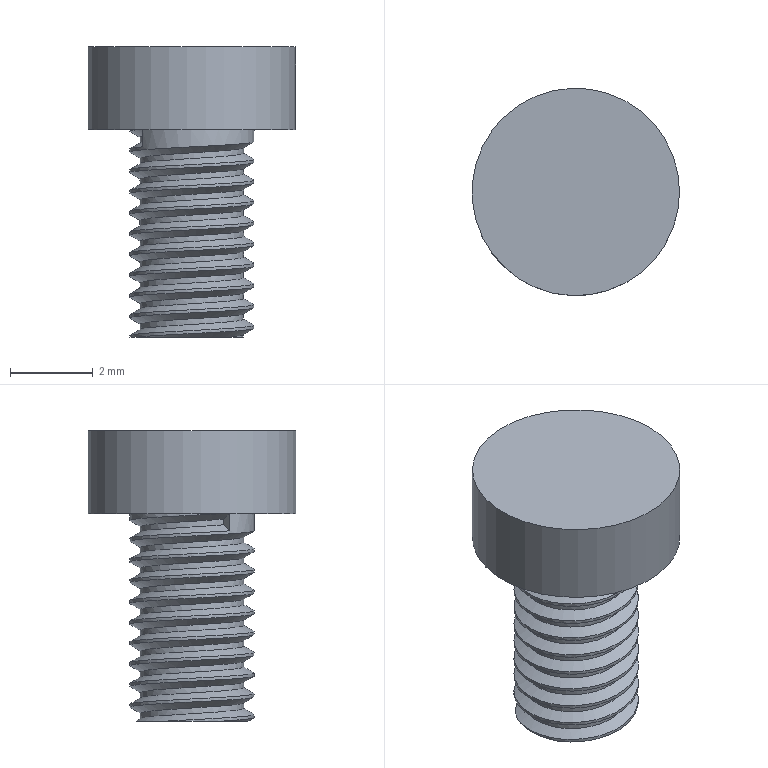Part | NX | features DATUM_CSYS 3, EXTRUDE 2, SKETCH 2, THREADS 1 | 1 solid | 10 faces | box 5 x 5 x 7 mm | volume 68.706 mm3 | plane 4 | cylinder 3 | spline 3 | commonest cylinder face diameters 2.5 x1 3 x1 5 x1